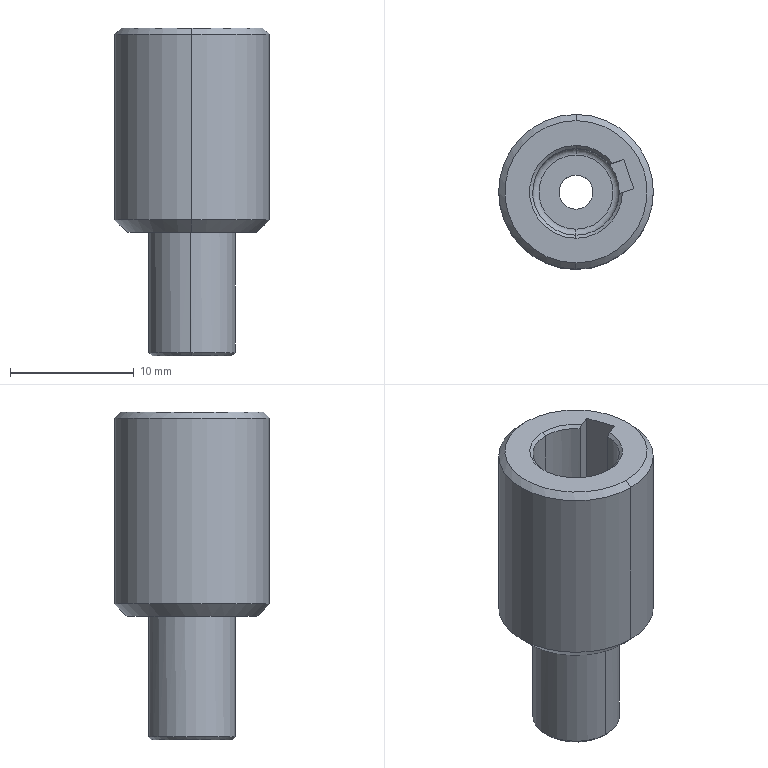Part | STEP file | 2026.6.15-Main Assembly图.sldasm-Part-128 | 1 solid | 37 faces | box 12.5 x 12.5 x 26.5 mm | volume 1705 mm3 | cylinder 13 | cone 11 | plane 11 | torus 2 | commonest cylinder face diameters 7 x5 2.5 x4 2.75 x2 12.5 x2
STEP:
#1=CARTESIAN_POINT('',(-1588.479,1436.224,3697.571));
#2=VERTEX_POINT('',#1);
#3=CARTESIAN_POINT('',(-1588.478,1436.235,3697.405));
#4=VERTEX_POINT('',#3);
#5=CARTESIAN_POINT('',(-1588.479,1436.224,3697.571));
#6=CARTESIAN_POINT('',(-1588.479,1436.224,3697.515));
#7=CARTESIAN_POINT('',(-1588.479,1436.228,3697.46));
#8=CARTESIAN_POINT('',(-1588.478,1436.235,3697.405));
#9=B_SPLINE_CURVE_WITH_KNOTS('',3,(#5,#6,#7,#8),.UNSPECIFIED.,.F.,.F.,(4,4),(0.,0.000165),.UNSPECIFIED.);
#10=EDGE_CURVE('',#2,#4,#9,.T.);
#11=ORIENTED_EDGE('',*,*,#10,.T.);
#12=CARTESIAN_POINT('',(-1589.685,1435.828,3697.405));
#13=VERTEX_POINT('',#12);
#14=CARTESIAN_POINT('',(-1589.685,1435.828,3697.405));
#15=DIRECTION('',(-0.9474,-0.3199,0.));
#16=VECTOR('',#15,1000.);
#17=LINE('',#14,#16);
#18=EDGE_CURVE('',#4,#13,#17,.T.);
#19=ORIENTED_EDGE('',*,*,#18,.T.);
#20=CARTESIAN_POINT('',(-1589.681,1435.818,3697.571));
#21=VERTEX_POINT('',#20);
#22=CARTESIAN_POINT('',(-1590.081,1437.002,3697.571));
#23=DIRECTION('',(0.9474,0.3199,0.));
#24=DIRECTION('',(-0.3171,0.9391,0.1324));
#25=AXIS2_PLACEMENT_3D('',#22,#23,#24);
#26=CIRCLE('',#25,1.25);
#27=EDGE_CURVE('',#21,#13,#26,.T.);
#28=ORIENTED_EDGE('',*,*,#27,.F.);
#29=CARTESIAN_POINT('',(-1589.681,1435.818,3697.571));
#30=DIRECTION('',(-0.9474,-0.3199,0.));
#31=VECTOR('',#30,1000.);
#32=LINE('',#29,#31);
#33=EDGE_CURVE('',#2,#21,#32,.T.);
#34=ORIENTED_EDGE('',*,*,#33,.F.);
#35=EDGE_LOOP('',(#11,#19,#28,#34));
#36=FACE_OUTER_BOUND('',#35,.T.);
#37=CARTESIAN_POINT('',(-1590.081,1437.002,3697.571));
#38=DIRECTION('',(-0.9474,-0.3199,0.));
#39=DIRECTION('',(0.3171,-0.9391,-0.1324));
#40=AXIS2_PLACEMENT_3D('',#37,#38,#39);
#41=CYLINDRICAL_SURFACE('',#40,1.25);
#42=ADVANCED_FACE('',(#36),#41,.F.);
#43=CARTESIAN_POINT('',(-1590.478,1438.176,3704.986));
#44=VERTEX_POINT('',#43);
#45=CARTESIAN_POINT('',(-1589.681,1435.818,3704.821));
#46=VERTEX_POINT('',#45);
#47=CARTESIAN_POINT('',(-1590.081,1437.002,3704.821));
#48=DIRECTION('',(0.9474,0.3199,0.));
#49=DIRECTION('',(-0.3171,0.9391,0.1324));
#50=AXIS2_PLACEMENT_3D('',#47,#48,#49);
#51=CIRCLE('',#50,1.25);
#52=EDGE_CURVE('',#44,#46,#51,.T.);
#53=ORIENTED_EDGE('',*,*,#52,.F.);
#54=CARTESIAN_POINT('',(-1589.271,1438.583,3704.986));
#55=VERTEX_POINT('',#54);
#56=CARTESIAN_POINT('',(-1590.478,1438.176,3704.986));
#57=DIRECTION('',(0.9474,0.3199,0.));
#58=VECTOR('',#57,1000.);
#59=LINE('',#56,#58);
#60=EDGE_CURVE('',#44,#55,#59,.T.);
#61=ORIENTED_EDGE('',*,*,#60,.T.);
#62=CARTESIAN_POINT('',(-1588.66,1437.482,3706.071));
#63=VERTEX_POINT('',#62);
#64=CARTESIAN_POINT('',(-1589.271,1438.583,3704.986));
#65=CARTESIAN_POINT('',(-1589.258,1438.567,3705.135));
#66=CARTESIAN_POINT('',(-1589.225,1438.527,3705.282));
#67=CARTESIAN_POINT('',(-1589.136,1438.409,3705.544));
#68=CARTESIAN_POINT('',(-1589.078,1438.328,3705.663));
#69=CARTESIAN_POINT('',(-1588.956,1438.134,3705.858));
#70=CARTESIAN_POINT('',(-1588.89,1438.019,3705.937));
#71=CARTESIAN_POINT('',(-1588.767,1437.765,3706.043));
#72=CARTESIAN_POINT('',(-1588.708,1437.625,3706.071));
#73=CARTESIAN_POINT('',(-1588.66,1437.482,3706.071));
#74=B_SPLINE_CURVE_WITH_KNOTS('',3,(#64,#65,#66,#67,#68,#69,#70,#71,#72,#73),.UNSPECIFIED.,.F.,.F.,(4,2,2,2,4),(0.000165,0.0006165,0.001068,0.001519,0.001971),.UNSPECIFIED.);
#75=EDGE_CURVE('',#55,#63,#74,.T.);
#76=ORIENTED_EDGE('',*,*,#75,.T.);
#77=CARTESIAN_POINT('',(-1588.479,1436.224,3704.821));
#78=VERTEX_POINT('',#77);
#79=CARTESIAN_POINT('',(-1588.66,1437.482,3706.071));
#80=CARTESIAN_POINT('',(-1588.634,1437.404,3706.071));
#81=CARTESIAN_POINT('',(-1588.61,1437.324,3706.062));
#82=CARTESIAN_POINT('',(-1588.569,1437.168,3706.03));
#83=CARTESIAN_POINT('',(-1588.552,1437.091,3706.006));
#84=CARTESIAN_POINT('',(-1588.509,1436.865,3705.911));
#85=CARTESIAN_POINT('',(-1588.493,1436.726,3705.819));
#86=CARTESIAN_POINT('',(-1588.481,1436.549,3705.647));
#87=CARTESIAN_POINT('',(-1588.478,1436.495,3705.585));
#88=CARTESIAN_POINT('',(-1588.476,1436.401,3705.45));
#89=CARTESIAN_POINT('',(-1588.476,1436.359,3705.377));
#90=CARTESIAN_POINT('',(-1588.477,1436.26,3705.152));
#91=CARTESIAN_POINT('',(-1588.479,1436.224,3704.987));
#92=CARTESIAN_POINT('',(-1588.479,1436.224,3704.821));
#93=B_SPLINE_CURVE_WITH_KNOTS('',3,(#79,#80,#81,#82,#83,#84,#85,#86,#87,#88,#89,#90,#91,#92),.UNSPECIFIED.,.F.,.F.,(4,2,2,2,2,2,4),(0.001971,0.002217,0.002463,0.002955,0.003201,0.003447,0.003939),.UNSPECIFIED.);
#94=EDGE_CURVE('',#63,#78,#93,.T.);
#95=ORIENTED_EDGE('',*,*,#94,.T.);
#96=CARTESIAN_POINT('',(-1589.681,1435.818,3704.821));
#97=DIRECTION('',(0.9474,0.3199,0.));
#98=VECTOR('',#97,1000.);
#99=LINE('',#96,#98);
#100=EDGE_CURVE('',#46,#78,#99,.T.);
#101=ORIENTED_EDGE('',*,*,#100,.F.);
#102=EDGE_LOOP('',(#53,#61,#76,#95,#101));
#103=FACE_OUTER_BOUND('',#102,.T.);
#104=CARTESIAN_POINT('',(-1590.081,1437.002,3704.821));
#105=DIRECTION('',(0.9474,0.3199,0.));
#106=DIRECTION('',(-0.3171,0.9391,0.1324));
#107=AXIS2_PLACEMENT_3D('',#104,#105,#106);
#108=CYLINDRICAL_SURFACE('',#107,1.25);
#109=ADVANCED_FACE('',(#103),#108,.F.);
#110=CARTESIAN_POINT('',(-1591.973,1439.862,3722.321));
#111=VERTEX_POINT('',#110);
#112=CARTESIAN_POINT('',(-1591.979,1432.862,3722.321));
#113=VERTEX_POINT('',#112);
#114=CARTESIAN_POINT('',(-1591.976,1436.362,3722.321));
#115=DIRECTION('',(0.,0.,1.));
#116=DIRECTION('',(0.0007664,1.,0.));
#117=AXIS2_PLACEMENT_3D('',#114,#115,#116);
#118=CIRCLE('',#117,3.5);
#119=EDGE_CURVE('',#111,#113,#118,.T.);
#120=ORIENTED_EDGE('',*,*,#119,.F.);
#121=CARTESIAN_POINT('',(-1591.973,1440.112,3722.571));
#122=VERTEX_POINT('',#121);
#123=CARTESIAN_POINT('',(-1591.973,1439.862,3722.321));
#124=DIRECTION('',(0.000542,0.7071,0.7071));
#125=VECTOR('',#124,1000.);
#126=LINE('',#123,#125);
#127=EDGE_CURVE('',#111,#122,#126,.T.);
#128=ORIENTED_EDGE('',*,*,#127,.T.);
#129=CARTESIAN_POINT('',(-1591.979,1432.612,3722.571));
#130=VERTEX_POINT('',#129);
#131=CARTESIAN_POINT('',(-1591.976,1436.362,3722.571));
#132=DIRECTION('',(0.,0.,-1.));
#133=DIRECTION('',(0.0007664,1.,0.));
#134=AXIS2_PLACEMENT_3D('',#131,#132,#133);
#135=CIRCLE('',#134,3.75);
#136=EDGE_CURVE('',#130,#122,#135,.T.);
#137=ORIENTED_EDGE('',*,*,#136,.F.);
#138=CARTESIAN_POINT('',(-1591.979,1432.862,3722.321));
#139=DIRECTION('',(-0.000542,-0.7071,0.7071));
#140=VECTOR('',#139,1000.);
#141=LINE('',#138,#140);
#142=EDGE_CURVE('',#113,#130,#141,.T.);
#143=ORIENTED_EDGE('',*,*,#142,.F.);
#144=EDGE_LOOP('',(#120,#128,#137,#143));
#145=FACE_OUTER_BOUND('',#144,.T.);
#146=CARTESIAN_POINT('',(-1591.976,1436.362,3722.321));
#147=DIRECTION('',(0.,0.,1.));
#148=DIRECTION('',(-0.0007664,-1.,0.));
#149=AXIS2_PLACEMENT_3D('',#146,#147,#148);
#150=CONICAL_SURFACE('',#149,3.5,0.7854);
#151=ADVANCED_FACE('',(#145),#150,.F.);
#152=CARTESIAN_POINT('',(-1588.479,1436.224,3722.321));
#153=VERTEX_POINT('',#152);
#154=CARTESIAN_POINT('',(-1591.976,1436.362,3722.321));
#155=DIRECTION('',(0.,0.,1.));
#156=DIRECTION('',(0.0007664,1.,0.));
#157=AXIS2_PLACEMENT_3D('',#154,#155,#156);
#158=CIRCLE('',#157,3.5);
#159=EDGE_CURVE('',#113,#153,#158,.T.);
#160=ORIENTED_EDGE('',*,*,#159,.F.);
#161=ORIENTED_EDGE('',*,*,#142,.T.);
#162=CARTESIAN_POINT('',(-1588.227,1436.309,3722.571));
#163=VERTEX_POINT('',#162);
#164=CARTESIAN_POINT('',(-1591.976,1436.362,3722.571));
#165=DIRECTION('',(0.,0.,-1.));
#166=DIRECTION('',(0.0007664,1.,0.));
#167=AXIS2_PLACEMENT_3D('',#164,#165,#166);
#168=CIRCLE('',#167,3.75);
#169=EDGE_CURVE('',#163,#130,#168,.T.);
#170=ORIENTED_EDGE('',*,*,#169,.F.);
#171=CARTESIAN_POINT('',(-1588.479,1436.224,3722.321));
#172=CARTESIAN_POINT('',(-1588.395,1436.252,3722.404));
#173=CARTESIAN_POINT('',(-1588.31,1436.281,3722.487));
#174=CARTESIAN_POINT('',(-1588.227,1436.309,3722.571));
#175=B_SPLINE_CURVE_WITH_KNOTS('',3,(#171,#172,#173,#174),.UNSPECIFIED.,.F.,.F.,(4,4),(0.,0.0003653),.UNSPECIFIED.);
#176=EDGE_CURVE('',#153,#163,#175,.T.);
#177=ORIENTED_EDGE('',*,*,#176,.F.);
#178=EDGE_LOOP('',(#160,#161,#170,#177));
#179=FACE_OUTER_BOUND('',#178,.T.);
#180=CARTESIAN_POINT('',(-1591.976,1436.362,3722.321));
#181=DIRECTION('',(0.,0.,1.));
#182=DIRECTION('',(-0.0007664,-1.,0.));
#183=AXIS2_PLACEMENT_3D('',#180,#181,#182);
#184=CONICAL_SURFACE('',#183,3.5,0.7854);
#185=ADVANCED_FACE('',(#179),#184,.F.);
#186=CARTESIAN_POINT('',(-1591.974,1439.612,3696.071));
#187=VERTEX_POINT('',#186);
#188=CARTESIAN_POINT('',(-1591.979,1433.112,3696.071));
#189=VERTEX_POINT('',#188);
#190=CARTESIAN_POINT('',(-1591.976,1436.362,3696.071));
#191=DIRECTION('',(0.,0.,-1.));
#192=DIRECTION('',(0.0007664,1.,0.));
#193=AXIS2_PLACEMENT_3D('',#190,#191,#192);
#194=CIRCLE('',#193,3.25);
#195=EDGE_CURVE('',#187,#189,#194,.T.);
#196=ORIENTED_EDGE('',*,*,#195,.F.);
#197=CARTESIAN_POINT('',(-1591.973,1439.862,3696.321));
#198=VERTEX_POINT('',#197);
#199=CARTESIAN_POINT('',(-1591.973,1439.862,3696.321));
#200=DIRECTION('',(0.000542,0.7071,0.7071));
#201=VECTOR('',#200,1000.);
#202=LINE('',#199,#201);
#203=EDGE_CURVE('',#187,#198,#202,.T.);
#204=ORIENTED_EDGE('',*,*,#203,.T.);
#205=CARTESIAN_POINT('',(-1591.84,1439.859,3696.321));
#206=VERTEX_POINT('',#205);
#207=CARTESIAN_POINT('',(-1591.976,1436.362,3696.321));
#208=DIRECTION('',(0.,0.,1.));
#209=DIRECTION('',(0.0007664,1.,0.));
#210=AXIS2_PLACEMENT_3D('',#207,#208,#209);
#211=CIRCLE('',#210,3.5);
#212=EDGE_CURVE('',#206,#198,#211,.T.);
#213=ORIENTED_EDGE('',*,*,#212,.F.);
#214=CARTESIAN_POINT('',(-1588.66,1437.482,3696.321));
#215=VERTEX_POINT('',#214);
#216=CARTESIAN_POINT('',(-1591.976,1436.362,3696.321));
#217=DIRECTION('',(0.,0.,1.));
#218=DIRECTION('',(0.0007664,1.,0.));
#219=AXIS2_PLACEMENT_3D('',#216,#217,#218);
#220=CIRCLE('',#219,3.5);
#221=EDGE_CURVE('',#215,#206,#220,.T.);
#222=ORIENTED_EDGE('',*,*,#221,.F.);
#223=CARTESIAN_POINT('',(-1591.979,1432.862,3696.321));
#224=VERTEX_POINT('',#223);
#225=CARTESIAN_POINT('',(-1591.976,1436.362,3696.321));
#226=DIRECTION('',(0.,0.,1.));
#227=DIRECTION('',(0.0007664,1.,0.));
#228=AXIS2_PLACEMENT_3D('',#225,#226,#227);
#229=CIRCLE('',#228,3.5);
#230=EDGE_CURVE('',#224,#215,#229,.T.);
#231=ORIENTED_EDGE('',*,*,#230,.F.);
#232=CARTESIAN_POINT('',(-1591.979,1432.862,3696.321));
#233=DIRECTION('',(-0.000542,-0.7071,0.7071));
#234=VECTOR('',#233,1000.);
#235=LINE('',#232,#234);
#236=EDGE_CURVE('',#189,#224,#235,.T.);
#237=ORIENTED_EDGE('',*,*,#236,.F.);
#238=EDGE_LOOP('',(#196,#204,#213,#222,#231,#237));
#239=FACE_OUTER_BOUND('',#238,.T.);
#240=CARTESIAN_POINT('',(-1591.976,1436.362,3696.321));
#241=DIRECTION('',(0.,0.,1.));
#242=DIRECTION('',(-0.0007664,-1.,0.));
#243=AXIS2_PLACEMENT_3D('',#240,#241,#242);
#244=CONICAL_SURFACE('',#243,3.5,0.7854);
#245=ADVANCED_FACE('',(#239),#244,.T.);
#246=CARTESIAN_POINT('',(-1591.977,1434.987,3696.321));
#247=VERTEX_POINT('',#246);
#248=CARTESIAN_POINT('',(-1591.975,1437.737,3696.321));
#249=VERTEX_POINT('',#248);
#250=CARTESIAN_POINT('',(-1591.976,1436.362,3696.321));
#251=DIRECTION('',(0.,0.,-1.));
#252=DIRECTION('',(0.0007664,1.,0.));
#253=AXIS2_PLACEMENT_3D('',#250,#251,#252);
#254=CIRCLE('',#253,1.375);
#255=EDGE_CURVE('',#247,#249,#254,.T.);
#256=ORIENTED_EDGE('',*,*,#255,.F.);
#257=CARTESIAN_POINT('',(-1591.977,1434.737,3696.071));
#258=VERTEX_POINT('',#257);
#259=CARTESIAN_POINT('',(-1591.977,1434.737,3696.071));
#260=DIRECTION('',(-0.000542,-0.7071,-0.7071));
#261=VECTOR('',#260,1000.);
#262=LINE('',#259,#261);
#263=EDGE_CURVE('',#247,#258,#262,.T.);
#264=ORIENTED_EDGE('',*,*,#263,.T.);
#265=CARTESIAN_POINT('',(-1591.975,1437.987,3696.071));
#266=VERTEX_POINT('',#265);
#267=CARTESIAN_POINT('',(-1591.976,1436.362,3696.071));
#268=DIRECTION('',(0.,0.,1.));
#269=DIRECTION('',(0.0007664,1.,0.));
#270=AXIS2_PLACEMENT_3D('',#267,#268,#269);
#271=CIRCLE('',#270,1.625);
#272=EDGE_CURVE('',#266,#258,#271,.T.);
#273=ORIENTED_EDGE('',*,*,#272,.F.);
#274=CARTESIAN_POINT('',(-1591.975,1437.987,3696.071));
#275=DIRECTION('',(0.000542,0.7071,-0.7071));
#276=VECTOR('',#275,1000.);
#277=LINE('',#274,#276);
#278=EDGE_CURVE('',#249,#266,#277,.T.);
#279=ORIENTED_EDGE('',*,*,#278,.F.);
#280=EDGE_LOOP('',(#256,#264,#273,#279));
#281=FACE_OUTER_BOUND('',#280,.T.);
#282=CARTESIAN_POINT('',(-1591.976,1436.362,3696.071));
#283=DIRECTION('',(0.,0.,-1.));
#284=DIRECTION('',(0.0007664,1.,0.));
#285=AXIS2_PLACEMENT_3D('',#282,#283,#284);
#286=CONICAL_SURFACE('',#285,1.625,0.7854);
#287=ADVANCED_FACE('',(#281),#286,.F.);
#288=CARTESIAN_POINT('',(-1591.981,1430.612,3722.571));
#289=VERTEX_POINT('',#288);
#290=CARTESIAN_POINT('',(-1591.972,1442.112,3722.571));
#291=VERTEX_POINT('',#290);
#292=CARTESIAN_POINT('',(-1591.976,1436.362,3722.571));
#293=DIRECTION('',(0.,0.,1.));
#294=DIRECTION('',(0.0007664,1.,0.));
#295=AXIS2_PLACEMENT_3D('',#292,#293,#294);
#296=CIRCLE('',#295,5.75);
#297=EDGE_CURVE('',#289,#291,#296,.T.);
#298=ORIENTED_EDGE('',*,*,#297,.F.);
#299=CARTESIAN_POINT('',(-1591.981,1430.112,3722.071));
#300=VERTEX_POINT('',#299);
#301=CARTESIAN_POINT('',(-1591.981,1430.112,3722.071));
#302=DIRECTION('',(-0.000542,-0.7071,-0.7071));
#303=VECTOR('',#302,1000.);
#304=LINE('',#301,#303);
#305=EDGE_CURVE('',#289,#300,#304,.T.);
#306=ORIENTED_EDGE('',*,*,#305,.T.);
#307=CARTESIAN_POINT('',(-1591.971,1442.612,3722.071));
#308=VERTEX_POINT('',#307);
#309=CARTESIAN_POINT('',(-1591.976,1436.362,3722.071));
#310=DIRECTION('',(0.,0.,-1.));
#311=DIRECTION('',(0.0007664,1.,0.));
#312=AXIS2_PLACEMENT_3D('',#309,#310,#311);
#313=CIRCLE('',#312,6.25);
#314=EDGE_CURVE('',#308,#300,#313,.T.);
#315=ORIENTED_EDGE('',*,*,#314,.F.);
#316=CARTESIAN_POINT('',(-1591.971,1442.612,3722.071));
#317=DIRECTION('',(0.000542,0.7071,-0.7071));
#318=VECTOR('',#317,1000.);
#319=LINE('',#316,#318);
#320=EDGE_CURVE('',#291,#308,#319,.T.);
#321=ORIENTED_EDGE('',*,*,#320,.F.);
#322=EDGE_LOOP('',(#298,#306,#315,#321));
#323=FACE_OUTER_BOUND('',#322,.T.);
#324=CARTESIAN_POINT('',(-1591.976,1436.362,3722.071));
#325=DIRECTION('',(0.,0.,-1.));
#326=DIRECTION('',(0.0007664,1.,0.));
#327=AXIS2_PLACEMENT_3D('',#324,#325,#326);
#328=CONICAL_SURFACE('',#327,6.25,0.7854);
#329=ADVANCED_FACE('',(#323),#328,.T.);
#330=CARTESIAN_POINT('',(-1591.972,1441.612,3706.071));
#331=VERTEX_POINT('',#330);
#332=CARTESIAN_POINT('',(-1591.98,1431.112,3706.071));
#333=VERTEX_POINT('',#332);
#334=CARTESIAN_POINT('',(-1591.976,1436.362,3706.071));
#335=DIRECTION('',(0.,0.,-1.));
#336=DIRECTION('',(0.0007664,1.,0.));
#337=AXIS2_PLACEMENT_3D('',#334,#335,#336);
#338=CIRCLE('',#337,5.25);
#339=EDGE_CURVE('',#331,#333,#338,.T.);
#340=ORIENTED_EDGE('',*,*,#339,.F.);
#341=CARTESIAN_POINT('',(-1591.971,1442.612,3707.071));
#342=VERTEX_POINT('',#341);
#343=CARTESIAN_POINT('',(-1591.972,1441.612,3706.071));
#344=DIRECTION('',(0.000542,0.7071,0.7071));
#345=VECTOR('',#344,1000.);
#346=LINE('',#343,#345);
#347=EDGE_CURVE('',#331,#342,#346,.T.);
#348=ORIENTED_EDGE('',*,*,#347,.T.);
#349=CARTESIAN_POINT('',(-1591.981,1430.112,3707.071));
#350=VERTEX_POINT('',#349);
#351=CARTESIAN_POINT('',(-1591.976,1436.362,3707.071));
#352=DIRECTION('',(0.,0.,1.));
#353=DIRECTION('',(0.0007664,1.,0.));
#354=AXIS2_PLACEMENT_3D('',#351,#352,#353);
#355=CIRCLE('',#354,6.25);
#356=EDGE_CURVE('',#350,#342,#355,.T.);
#357=ORIENTED_EDGE('',*,*,#356,.F.);
#358=CARTESIAN_POINT('',(-1591.98,1431.112,3706.071));
#359=DIRECTION('',(-0.000542,-0.7071,0.7071));
#360=VECTOR('',#359,1000.);
#361=LINE('',#358,#360);
#362=EDGE_CURVE('',#333,#350,#361,.T.);
#363=ORIENTED_EDGE('',*,*,#362,.F.);
#364=EDGE_LOOP('',(#340,#348,#357,#363));
#365=FACE_OUTER_BOUND('',#364,.T.);
#366=CARTESIAN_POINT('',(-1591.976,1436.362,3706.071));
#367=DIRECTION('',(0.,0.,1.));
#368=DIRECTION('',(-0.0007664,-1.,0.));
#369=AXIS2_PLACEMENT_3D('',#366,#367,#368);
#370=CONICAL_SURFACE('',#369,5.25,0.7854);
#371=ADVANCED_FACE('',(#365),#370,.T.);
#372=ORIENTED_EDGE('',*,*,#255,.T.);
#373=CARTESIAN_POINT('',(-1591.975,1437.737,3708.571));
#374=VERTEX_POINT('',#373);
#375=CARTESIAN_POINT('',(-1591.975,1437.737,3693.071));
#376=DIRECTION('',(0.,0.,1.));
#377=VECTOR('',#376,1000.);
#378=LINE('',#375,#377);
#379=EDGE_CURVE('',#249,#374,#378,.T.);
#380=ORIENTED_EDGE('',*,*,#379,.T.);
#381=CARTESIAN_POINT('',(-1591.977,1434.987,3708.571));
#382=VERTEX_POINT('',#381);
#383=CARTESIAN_POINT('',(-1591.976,1436.362,3708.571));
#384=DIRECTION('',(0.,0.,-1.));
#385=DIRECTION('',(-0.0007664,-1.,0.));
#386=AXIS2_PLACEMENT_3D('',#383,#384,#385);
#387=CIRCLE('',#386,1.375);
#388=EDGE_CURVE('',#382,#374,#387,.T.);
#389=ORIENTED_EDGE('',*,*,#388,.F.);
#390=CARTESIAN_POINT('',(-1591.977,1434.987,3693.071));
#391=DIRECTION('',(0.,0.,1.));
#392=VECTOR('',#391,1000.);
#393=LINE('',#390,#392);
#394=EDGE_CURVE('',#247,#382,#393,.T.);
#395=ORIENTED_EDGE('',*,*,#394,.F.);
#396=EDGE_LOOP('',(#372,#380,#389,#395));
#397=FACE_OUTER_BOUND('',#396,.T.);
#398=CARTESIAN_POINT('',(-1591.976,1436.362,3693.071));
#399=DIRECTION('',(0.,0.,1.));
#400=DIRECTION('',(-0.0007664,-1.,0.));
#401=AXIS2_PLACEMENT_3D('',#398,#399,#400);
#402=CYLINDRICAL_SURFACE('',#401,1.375);
#403=ADVANCED_FACE('',(#397),#402,.F.);
#404=CARTESIAN_POINT('',(-1591.974,1439.362,3708.571));
#405=VERTEX_POINT('',#404);
#406=CARTESIAN_POINT('',(-1591.978,1433.362,3708.571));
#407=VERTEX_POINT('',#406);
#408=CARTESIAN_POINT('',(-1591.976,1436.362,3708.571));
#409=DIRECTION('',(0.,0.,1.));
#410=DIRECTION('',(-0.0007664,-1.,0.));
#411=AXIS2_PLACEMENT_3D('',#408,#409,#410);
#412=CIRCLE('',#411,3.);
#413=EDGE_CURVE('',#405,#407,#412,.T.);
#414=ORIENTED_EDGE('',*,*,#413,.F.);
#415=CARTESIAN_POINT('',(-1591.973,1439.862,3709.071));
#416=VERTEX_POINT('',#415);
#417=CARTESIAN_POINT('',(-1591.974,1439.362,3709.071));
#418=DIRECTION('',(1.,-0.0007664,0.));
#419=DIRECTION('',(0.0007664,1.,0.));
#420=AXIS2_PLACEMENT_3D('',#417,#418,#419);
#421=CIRCLE('',#420,0.5);
#422=EDGE_CURVE('',#405,#416,#421,.T.);
#423=ORIENTED_EDGE('',*,*,#422,.T.);
#424=CARTESIAN_POINT('',(-1591.979,1432.862,3709.071));
#425=VERTEX_POINT('',#424);
#426=CARTESIAN_POINT('',(-1591.976,1436.362,3709.071));
#427=DIRECTION('',(0.,0.,-1.));
#428=DIRECTION('',(-0.0007664,-1.,0.));
#429=AXIS2_PLACEMENT_3D('',#426,#427,#428);
#430=CIRCLE('',#429,3.5);
#431=EDGE_CURVE('',#425,#416,#430,.T.);
#432=ORIENTED_EDGE('',*,*,#431,.F.);
#433=CARTESIAN_POINT('',(-1591.978,1433.362,3709.071));
#434=DIRECTION('',(-1.,0.0007664,0.));
#435=DIRECTION('',(-0.0007664,-1.,0.));
#436=AXIS2_PLACEMENT_3D('',#433,#434,#435);
#437=CIRCLE('',#436,0.5);
#438=EDGE_CURVE('',#407,#425,#437,.T.);
#439=ORIENTED_EDGE('',*,*,#438,.F.);
#440=EDGE_LOOP('',(#414,#423,#432,#439));
#441=FACE_OUTER_BOUND('',#440,.T.);
#442=CARTESIAN_POINT('',(-1591.976,1436.362,3709.071));
#443=DIRECTION('',(0.,0.,1.));
#444=DIRECTION('',(-0.0007664,-1.,0.));
#445=AXIS2_PLACEMENT_3D('',#442,#443,#444);
#446=TOROIDAL_SURFACE('',#445,3.,0.5);
#447=ADVANCED_FACE('',(#441),#446,.F.);
#448=ORIENTED_EDGE('',*,*,#431,.T.);
#449=CARTESIAN_POINT('',(-1591.973,1439.862,3708.571));
#450=DIRECTION('',(0.,0.,1.));
#451=VECTOR('',#450,1000.);
#452=LINE('',#449,#451);
#453=EDGE_CURVE('',#416,#111,#452,.T.);
#454=ORIENTED_EDGE('',*,*,#453,.T.);
#455=ORIENTED_EDGE('',*,*,#119,.T.);
#456=CARTESIAN_POINT('',(-1591.979,1432.862,3708.571));
#457=DIRECTION('',(0.,0.,1.));
#458=VECTOR('',#457,1000.);
#459=LINE('',#456,#458);
#460=EDGE_CURVE('',#425,#113,#459,.T.);
#461=ORIENTED_EDGE('',*,*,#460,.F.);
#462=EDGE_LOOP('',(#448,#454,#455,#461));
#463=FACE_OUTER_BOUND('',#462,.T.);
#464=CARTESIAN_POINT('',(-1591.976,1436.362,3708.571));
#465=DIRECTION('',(0.,0.,1.));
#466=DIRECTION('',(-0.0007664,-1.,0.));
#467=AXIS2_PLACEMENT_3D('',#464,#465,#466);
#468=CYLINDRICAL_SURFACE('',#467,3.5);
#469=ADVANCED_FACE('',(#463),#468,.F.);
#470=ORIENTED_EDGE('',*,*,#356,.T.);
#471=CARTESIAN_POINT('',(-1591.971,1442.612,3706.071));
#472=DIRECTION('',(0.,0.,1.));
#473=VECTOR('',#472,1000.);
#474=LINE('',#471,#473);
#475=EDGE_CURVE('',#342,#308,#474,.T.);
#476=ORIENTED_EDGE('',*,*,#475,.T.);
#477=ORIENTED_EDGE('',*,*,#314,.T.);
#478=CARTESIAN_POINT('',(-1591.981,1430.112,3706.071));
#479=DIRECTION('',(0.,0.,1.));
#480=VECTOR('',#479,1000.);
#481=LINE('',#478,#480);
#482=EDGE_CURVE('',#350,#300,#481,.T.);
#483=ORIENTED_EDGE('',*,*,#482,.F.);
#484=EDGE_LOOP('',(#470,#476,#477,#483));
#485=FACE_OUTER_BOUND('',#484,.T.);
#486=CARTESIAN_POINT('',(-1591.976,1436.362,3706.071));
#487=DIRECTION('',(0.,0.,1.));
#488=DIRECTION('',(-0.0007664,-1.,0.));
#489=AXIS2_PLACEMENT_3D('',#486,#487,#488);
#490=CYLINDRICAL_SURFACE('',#489,6.25);
#491=ADVANCED_FACE('',(#485),#490,.T.);
#492=CARTESIAN_POINT('',(-1592.112,1432.865,3706.071));
#493=VERTEX_POINT('',#492);
#494=CARTESIAN_POINT('',(-1591.976,1436.362,3706.071));
#495=DIRECTION('',(0.,0.,-1.));
#496=DIRECTION('',(0.03892,0.9992,0.));
#497=AXIS2_PLACEMENT_3D('',#494,#495,#496);
#498=CIRCLE('',#497,3.5);
#499=EDGE_CURVE('',#63,#493,#498,.T.);
#500=ORIENTED_EDGE('',*,*,#499,.T.);
#501=CARTESIAN_POINT('',(-1592.112,1432.865,3696.321));
#502=VERTEX_POINT('',#501);
#503=CARTESIAN_POINT('',(-1592.112,1432.865,3706.071));
#504=DIRECTION('',(0.,0.,-1.));
#505=VECTOR('',#504,1000.);
#506=LINE('',#503,#505);
#507=EDGE_CURVE('',#493,#502,#506,.T.);
#508=ORIENTED_EDGE('',*,*,#507,.T.);
#509=CARTESIAN_POINT('',(-1591.976,1436.362,3696.321));
#510=DIRECTION('',(0.,0.,1.));
#511=DIRECTION('',(0.0007664,1.,0.));
#512=AXIS2_PLACEMENT_3D('',#509,#510,#511);
#513=CIRCLE('',#512,3.5);
#514=EDGE_CURVE('',#502,#224,#513,.T.);
#515=ORIENTED_EDGE('',*,*,#514,.T.);
#516=ORIENTED_EDGE('',*,*,#230,.T.);
#517=CARTESIAN_POINT('',(-1588.478,1436.235,3697.405));
#518=CARTESIAN_POINT('',(-1588.478,1436.257,3697.256));
#519=CARTESIAN_POINT('',(-1588.476,1436.308,3697.11));
#520=CARTESIAN_POINT('',(-1588.477,1436.456,3696.848));
#521=CARTESIAN_POINT('',(-1588.48,1436.555,3696.729));
#522=CARTESIAN_POINT('',(-1588.5,1436.784,3696.533));
#523=CARTESIAN_POINT('',(-1588.517,1436.915,3696.455));
#524=CARTESIAN_POINT('',(-1588.573,1437.192,3696.349));
#525=CARTESIAN_POINT('',(-1588.612,1437.339,3696.321));
#526=CARTESIAN_POINT('',(-1588.66,1437.482,3696.321));
#527=B_SPLINE_CURVE_WITH_KNOTS('',3,(#517,#518,#519,#520,#521,#522,#523,#524,#525,#526),.UNSPECIFIED.,.F.,.F.,(4,2,2,2,4),(0.000165,0.0006165,0.001068,0.001519,0.001971),.UNSPECIFIED.);
#528=EDGE_CURVE('',#4,#215,#527,.T.);
#529=ORIENTED_EDGE('',*,*,#528,.F.);
#530=ORIENTED_EDGE('',*,*,#10,.F.);
#531=CARTESIAN_POINT('',(-1588.479,1436.224,3706.071));
#532=DIRECTION('',(0.,0.,-1.));
#533=VECTOR('',#532,1000.);
#534=LINE('',#531,#533);
#535=EDGE_CURVE('',#78,#2,#534,.T.);
#536=ORIENTED_EDGE('',*,*,#535,.F.);
#537=ORIENTED_EDGE('',*,*,#94,.F.);
#538=EDGE_LOOP('',(#500,#508,#515,#516,#529,#530,#536,#537));
#539=FACE_OUTER_BOUND('',#538,.T.);
#540=CARTESIAN_POINT('',(-1591.976,1436.362,3706.071));
#541=DIRECTION('',(0.,0.,-1.));
#542=DIRECTION('',(0.03892,0.9992,0.));
#543=AXIS2_PLACEMENT_3D('',#540,#541,#542);
#544=CYLINDRICAL_SURFACE('',#543,3.5);
#545=ADVANCED_FACE('',(#539),#544,.T.);
#546=ORIENTED_EDGE('',*,*,#507,.F.);
#547=CARTESIAN_POINT('',(-1591.84,1439.859,3706.071));
#548=VERTEX_POINT('',#547);
#549=CARTESIAN_POINT('',(-1591.976,1436.362,3706.071));
#550=DIRECTION('',(0.,0.,-1.));
#551=DIRECTION('',(0.03892,0.9992,0.));
#552=AXIS2_PLACEMENT_3D('',#549,#550,#551);
#553=CIRCLE('',#552,3.5);
#554=EDGE_CURVE('',#493,#548,#553,.T.);
#555=ORIENTED_EDGE('',*,*,#554,.T.);
#556=CARTESIAN_POINT('',(-1591.84,1439.859,3706.071));
#557=DIRECTION('',(0.,0.,-1.));
#558=VECTOR('',#557,1000.);
#559=LINE('',#556,#558);
#560=EDGE_CURVE('',#548,#206,#559,.T.);
#561=ORIENTED_EDGE('',*,*,#560,.T.);
#562=ORIENTED_EDGE('',*,*,#212,.T.);
#563=CARTESIAN_POINT('',(-1591.976,1436.362,3696.321));
#564=DIRECTION('',(0.,0.,1.));
#565=DIRECTION('',(0.0007664,1.,0.));
#566=AXIS2_PLACEMENT_3D('',#563,#564,#565);
#567=CIRCLE('',#566,3.5);
#568=EDGE_CURVE('',#198,#502,#567,.T.);
#569=ORIENTED_EDGE('',*,*,#568,.T.);
#570=EDGE_LOOP('',(#546,#555,#561,#562,#569));
#571=FACE_OUTER_BOUND('',#570,.T.);
#572=CARTESIAN_POINT('',(-1591.976,1436.362,3706.071));
#573=DIRECTION('',(0.,0.,-1.));
#574=DIRECTION('',(0.03892,0.9992,0.));
#575=AXIS2_PLACEMENT_3D('',#572,#573,#574);
#576=CYLINDRICAL_SURFACE('',#575,3.5);
#577=ADVANCED_FACE('',(#571),#576,.T.);
#578=ORIENTED_EDGE('',*,*,#272,.T.);
#579=CARTESIAN_POINT('',(-1591.976,1436.362,3696.071));
#580=DIRECTION('',(0.,0.,1.));
#581=DIRECTION('',(0.0007664,1.,0.));
#582=AXIS2_PLACEMENT_3D('',#579,#580,#581);
#583=CIRCLE('',#582,1.625);
#584=EDGE_CURVE('',#258,#266,#583,.T.);
#585=ORIENTED_EDGE('',*,*,#584,.T.);
#586=EDGE_LOOP('',(#578,#585));
#587=FACE_BOUND('',#586,.T.);
#588=CARTESIAN_POINT('',(-1591.976,1436.362,3696.071));
#589=DIRECTION('',(0.,0.,-1.));
#590=DIRECTION('',(0.0007664,1.,0.));
#591=AXIS2_PLACEMENT_3D('',#588,#589,#590);
#592=CIRCLE('',#591,3.25);
#593=EDGE_CURVE('',#189,#187,#592,.T.);
#594=ORIENTED_EDGE('',*,*,#593,.T.);
#595=ORIENTED_EDGE('',*,*,#195,.T.);
#596=EDGE_LOOP('',(#594,#595));
#597=FACE_OUTER_BOUND('',#596,.T.);
#598=CARTESIAN_POINT('',(-1591.976,1436.362,3696.071));
#599=DIRECTION('',(0.,0.,-1.));
#600=DIRECTION('',(0.0007664,1.,0.));
#601=AXIS2_PLACEMENT_3D('',#598,#599,#600);
#602=PLANE('',#601);
#603=ADVANCED_FACE('',(#587,#597),#602,.T.);
#604=ORIENTED_EDGE('',*,*,#560,.F.);
#605=CARTESIAN_POINT('',(-1591.976,1436.362,3706.071));
#606=DIRECTION('',(0.,0.,-1.));
#607=DIRECTION('',(0.03892,0.9992,0.));
#608=AXIS2_PLACEMENT_3D('',#605,#606,#607);
#609=CIRCLE('',#608,3.5);
#610=EDGE_CURVE('',#548,#63,#609,.T.);
#611=ORIENTED_EDGE('',*,*,#610,.T.);
#612=ORIENTED_EDGE('',*,*,#75,.F.);
#613=CARTESIAN_POINT('',(-1589.279,1438.592,3704.821));
#614=VERTEX_POINT('',#613);
#615=CARTESIAN_POINT('',(-1589.279,1438.592,3704.821));
#616=CARTESIAN_POINT('',(-1589.279,1438.592,3704.877));
#617=CARTESIAN_POINT('',(-1589.276,1438.589,3704.932));
#618=CARTESIAN_POINT('',(-1589.271,1438.583,3704.986));
#619=B_SPLINE_CURVE_WITH_KNOTS('',3,(#615,#616,#617,#618),.UNSPECIFIED.,.F.,.F.,(4,4),(0.,0.000165),.UNSPECIFIED.);
#620=EDGE_CURVE('',#614,#55,#619,.T.);
#621=ORIENTED_EDGE('',*,*,#620,.F.);
#622=CARTESIAN_POINT('',(-1589.279,1438.592,3697.571));
#623=VERTEX_POINT('',#622);
#624=CARTESIAN_POINT('',(-1589.279,1438.592,3706.071));
#625=DIRECTION('',(0.,0.,1.));
#626=VECTOR('',#625,1000.);
#627=LINE('',#624,#626);
#628=EDGE_CURVE('',#623,#614,#627,.T.);
#629=ORIENTED_EDGE('',*,*,#628,.F.);
#630=CARTESIAN_POINT('',(-1588.66,1437.482,3696.321));
#631=CARTESIAN_POINT('',(-1588.686,1437.56,3696.321));
#632=CARTESIAN_POINT('',(-1588.716,1437.638,3696.329));
#633=CARTESIAN_POINT('',(-1588.778,1437.787,3696.361));
#634=CARTESIAN_POINT('',(-1588.811,1437.858,3696.385));
#635=CARTESIAN_POINT('',(-1588.914,1438.064,3696.48));
#636=CARTESIAN_POINT('',(-1588.985,1438.184,3696.572));
#637=CARTESIAN_POINT('',(-1589.083,1438.333,3696.745));
#638=CARTESIAN_POINT('',(-1589.114,1438.377,3696.807));
#639=CARTESIAN_POINT('',(-1589.169,1438.453,3696.942));
#640=CARTESIAN_POINT('',(-1589.194,1438.486,3697.015));
#641=CARTESIAN_POINT('',(-1589.255,1438.565,3697.24));
#642=CARTESIAN_POINT('',(-1589.279,1438.592,3697.404));
#643=CARTESIAN_POINT('',(-1589.279,1438.592,3697.571));
#644=B_SPLINE_CURVE_WITH_KNOTS('',3,(#630,#631,#632,#633,#634,#635,#636,#637,#638,#639,#640,#641,#642,#643),.UNSPECIFIED.,.F.,.F.,(4,2,2,2,2,2,4),(0.001971,0.002217,0.002463,0.002955,0.003201,0.003447,0.003939),.UNSPECIFIED.);
#645=EDGE_CURVE('',#215,#623,#644,.T.);
#646=ORIENTED_EDGE('',*,*,#645,.F.);
#647=ORIENTED_EDGE('',*,*,#221,.T.);
#648=EDGE_LOOP('',(#604,#611,#612,#621,#629,#646,#647));
#649=FACE_OUTER_BOUND('',#648,.T.);
#650=CARTESIAN_POINT('',(-1591.976,1436.362,3706.071));
#651=DIRECTION('',(0.,0.,-1.));
#652=DIRECTION('',(0.03892,0.9992,0.));
#653=AXIS2_PLACEMENT_3D('',#650,#651,#652);
#654=CYLINDRICAL_SURFACE('',#653,3.5);
#655=ADVANCED_FACE('',(#649),#654,.T.);
#656=ORIENTED_EDGE('',*,*,#475,.F.);
#657=CARTESIAN_POINT('',(-1591.976,1436.362,3707.071));
#658=DIRECTION('',(0.,0.,1.));
#659=DIRECTION('',(0.0007664,1.,0.));
#660=AXIS2_PLACEMENT_3D('',#657,#658,#659);
#661=CIRCLE('',#660,6.25);
#662=EDGE_CURVE('',#342,#350,#661,.T.);
#663=ORIENTED_EDGE('',*,*,#662,.T.);
#664=ORIENTED_EDGE('',*,*,#482,.T.);
#665=CARTESIAN_POINT('',(-1591.976,1436.362,3722.071));
#666=DIRECTION('',(0.,0.,-1.));
#667=DIRECTION('',(0.0007664,1.,0.));
#668=AXIS2_PLACEMENT_3D('',#665,#666,#667);
#669=CIRCLE('',#668,6.25);
#670=EDGE_CURVE('',#300,#308,#669,.T.);
#671=ORIENTED_EDGE('',*,*,#670,.T.);
#672=EDGE_LOOP('',(#656,#663,#664,#671));
#673=FACE_OUTER_BOUND('',#672,.T.);
#674=CARTESIAN_POINT('',(-1591.976,1436.362,3706.071));
#675=DIRECTION('',(0.,0.,1.));
#676=DIRECTION('',(-0.0007664,-1.,0.));
#677=AXIS2_PLACEMENT_3D('',#674,#675,#676);
#678=CYLINDRICAL_SURFACE('',#677,6.25);
#679=ADVANCED_FACE('',(#673),#678,.T.);
#680=CARTESIAN_POINT('',(-1591.976,1436.362,3706.071));
#681=DIRECTION('',(0.,0.,-1.));
#682=DIRECTION('',(0.0007664,1.,0.));
#683=AXIS2_PLACEMENT_3D('',#680,#681,#682);
#684=CIRCLE('',#683,5.25);
#685=EDGE_CURVE('',#333,#331,#684,.T.);
#686=ORIENTED_EDGE('',*,*,#685,.T.);
#687=ORIENTED_EDGE('',*,*,#339,.T.);
#688=EDGE_LOOP('',(#686,#687));
#689=FACE_OUTER_BOUND('',#688,.T.);
#690=ORIENTED_EDGE('',*,*,#499,.F.);
#691=ORIENTED_EDGE('',*,*,#610,.F.);
#692=ORIENTED_EDGE('',*,*,#554,.F.);
#693=EDGE_LOOP('',(#690,#691,#692));
#694=FACE_BOUND('',#693,.T.);
#695=CARTESIAN_POINT('',(-1591.976,1436.362,3706.071));
#696=DIRECTION('',(0.,0.,-1.));
#697=DIRECTION('',(0.0007664,1.,0.));
#698=AXIS2_PLACEMENT_3D('',#695,#696,#697);
#699=PLANE('',#698);
#700=ADVANCED_FACE('',(#689,#694),#699,.T.);
#701=CARTESIAN_POINT('',(-1591.976,1436.362,3722.571));
#702=DIRECTION('',(0.,0.,1.));
#703=DIRECTION('',(0.0007664,1.,0.));
#704=AXIS2_PLACEMENT_3D('',#701,#702,#703);
#705=CIRCLE('',#704,5.75);
#706=EDGE_CURVE('',#291,#289,#705,.T.);
#707=ORIENTED_EDGE('',*,*,#706,.T.);
#708=ORIENTED_EDGE('',*,*,#297,.T.);
#709=EDGE_LOOP('',(#707,#708));
#710=FACE_OUTER_BOUND('',#709,.T.);
#711=CARTESIAN_POINT('',(-1587.313,1436.617,3722.571));
#712=VERTEX_POINT('',#711);
#713=CARTESIAN_POINT('',(-1587.313,1436.617,3722.571));
#714=DIRECTION('',(-0.9474,-0.3199,0.));
#715=VECTOR('',#714,1000.);
#716=LINE('',#713,#715);
#717=EDGE_CURVE('',#712,#163,#716,.T.);
#718=ORIENTED_EDGE('',*,*,#717,.T.);
#719=ORIENTED_EDGE('',*,*,#169,.T.);
#720=ORIENTED_EDGE('',*,*,#136,.T.);
#721=CARTESIAN_POINT('',(-1589.026,1438.677,3722.571));
#722=VERTEX_POINT('',#721);
#723=CARTESIAN_POINT('',(-1591.976,1436.362,3722.571));
#724=DIRECTION('',(0.,0.,-1.));
#725=DIRECTION('',(0.0007664,1.,0.));
#726=AXIS2_PLACEMENT_3D('',#723,#724,#725);
#727=CIRCLE('',#726,3.75);
#728=EDGE_CURVE('',#122,#722,#727,.T.);
#729=ORIENTED_EDGE('',*,*,#728,.T.);
#730=CARTESIAN_POINT('',(-1588.113,1438.986,3722.571));
#731=VERTEX_POINT('',#730);
#732=CARTESIAN_POINT('',(-1589.279,1438.592,3722.571));
#733=DIRECTION('',(0.9474,0.3199,0.));
#734=VECTOR('',#733,1000.);
#735=LINE('',#732,#734);
#736=EDGE_CURVE('',#722,#731,#735,.T.);
#737=ORIENTED_EDGE('',*,*,#736,.T.);
#738=CARTESIAN_POINT('',(-1588.113,1438.986,3722.571));
#739=DIRECTION('',(0.3199,-0.9474,0.));
#740=VECTOR('',#739,1000.);
#741=LINE('',#738,#740);
#742=EDGE_CURVE('',#731,#712,#741,.T.);
#743=ORIENTED_EDGE('',*,*,#742,.T.);
#744=EDGE_LOOP('',(#718,#719,#720,#729,#737,#743));
#745=FACE_BOUND('',#744,.T.);
#746=CARTESIAN_POINT('',(-1591.976,1436.362,3722.571));
#747=DIRECTION('',(0.,0.,-1.));
#748=DIRECTION('',(0.0007664,1.,0.));
#749=AXIS2_PLACEMENT_3D('',#746,#747,#748);
#750=PLANE('',#749);
#751=ADVANCED_FACE('',(#710,#745),#750,.F.);
#752=ORIENTED_EDGE('',*,*,#453,.F.);
#753=CARTESIAN_POINT('',(-1591.976,1436.362,3709.071));
#754=DIRECTION('',(0.,0.,-1.));
#755=DIRECTION('',(-0.0007664,-1.,0.));
#756=AXIS2_PLACEMENT_3D('',#753,#754,#755);
#757=CIRCLE('',#756,3.5);
#758=EDGE_CURVE('',#416,#425,#757,.T.);
#759=ORIENTED_EDGE('',*,*,#758,.T.);
#760=ORIENTED_EDGE('',*,*,#460,.T.);
#761=ORIENTED_EDGE('',*,*,#159,.T.);
#762=CARTESIAN_POINT('',(-1588.479,1436.224,3709.571));
#763=VERTEX_POINT('',#762);
#764=CARTESIAN_POINT('',(-1588.479,1436.224,3709.571));
#765=DIRECTION('',(0.,0.,1.));
#766=VECTOR('',#765,1000.);
#767=LINE('',#764,#766);
#768=EDGE_CURVE('',#763,#153,#767,.T.);
#769=ORIENTED_EDGE('',*,*,#768,.F.);
#770=CARTESIAN_POINT('',(-1589.279,1438.592,3709.571));
#771=VERTEX_POINT('',#770);
#772=CARTESIAN_POINT('',(-1591.976,1436.362,3709.571));
#773=DIRECTION('',(0.,0.,1.));
#774=DIRECTION('',(-0.3199,0.9474,0.));
#775=AXIS2_PLACEMENT_3D('',#772,#773,#774);
#776=CIRCLE('',#775,3.5);
#777=EDGE_CURVE('',#763,#771,#776,.T.);
#778=ORIENTED_EDGE('',*,*,#777,.T.);
#779=CARTESIAN_POINT('',(-1589.279,1438.592,3722.321));
#780=VERTEX_POINT('',#779);
#781=CARTESIAN_POINT('',(-1589.279,1438.592,3709.571));
#782=DIRECTION('',(0.,0.,1.));
#783=VECTOR('',#782,1000.);
#784=LINE('',#781,#783);
#785=EDGE_CURVE('',#771,#780,#784,.T.);
#786=ORIENTED_EDGE('',*,*,#785,.T.);
#787=CARTESIAN_POINT('',(-1591.976,1436.362,3722.321));
#788=DIRECTION('',(0.,0.,1.));
#789=DIRECTION('',(0.0007664,1.,0.));
#790=AXIS2_PLACEMENT_3D('',#787,#788,#789);
#791=CIRCLE('',#790,3.5);
#792=EDGE_CURVE('',#780,#111,#791,.T.);
#793=ORIENTED_EDGE('',*,*,#792,.T.);
#794=EDGE_LOOP('',(#752,#759,#760,#761,#769,#778,#786,#793));
#795=FACE_OUTER_BOUND('',#794,.T.);
#796=CARTESIAN_POINT('',(-1591.976,1436.362,3708.571));
#797=DIRECTION('',(0.,0.,1.));
#798=DIRECTION('',(-0.0007664,-1.,0.));
#799=AXIS2_PLACEMENT_3D('',#796,#797,#798);
#800=CYLINDRICAL_SURFACE('',#799,3.5);
#801=ADVANCED_FACE('',(#795),#800,.F.);
#802=ORIENTED_EDGE('',*,*,#388,.T.);
#803=CARTESIAN_POINT('',(-1591.976,1436.362,3708.571));
#804=DIRECTION('',(0.,0.,-1.));
#805=DIRECTION('',(-0.0007664,-1.,0.));
#806=AXIS2_PLACEMENT_3D('',#803,#804,#805);
#807=CIRCLE('',#806,1.375);
#808=EDGE_CURVE('',#374,#382,#807,.T.);
#809=ORIENTED_EDGE('',*,*,#808,.T.);
#810=EDGE_LOOP('',(#802,#809));
#811=FACE_BOUND('',#810,.T.);
#812=CARTESIAN_POINT('',(-1591.976,1436.362,3708.571));
#813=DIRECTION('',(0.,0.,1.));
#814=DIRECTION('',(-0.0007664,-1.,0.));
#815=AXIS2_PLACEMENT_3D('',#812,#813,#814);
#816=CIRCLE('',#815,3.);
#817=EDGE_CURVE('',#407,#405,#816,.T.);
#818=ORIENTED_EDGE('',*,*,#817,.T.);
#819=ORIENTED_EDGE('',*,*,#413,.T.);
#820=EDGE_LOOP('',(#818,#819));
#821=FACE_OUTER_BOUND('',#820,.T.);
#822=CARTESIAN_POINT('',(-1591.976,1436.362,3708.571));
#823=DIRECTION('',(0.,0.,1.));
#824=DIRECTION('',(-0.0007664,-1.,0.));
#825=AXIS2_PLACEMENT_3D('',#822,#823,#824);
#826=PLANE('',#825);
#827=ADVANCED_FACE('',(#811,#821),#826,.T.);
#828=ORIENTED_EDGE('',*,*,#736,.F.);
#829=CARTESIAN_POINT('',(-1589.026,1438.677,3722.571));
#830=CARTESIAN_POINT('',(-1589.11,1438.649,3722.487));
#831=CARTESIAN_POINT('',(-1589.194,1438.621,3722.404));
#832=CARTESIAN_POINT('',(-1589.279,1438.592,3722.321));
#833=B_SPLINE_CURVE_WITH_KNOTS('',3,(#829,#830,#831,#832),.UNSPECIFIED.,.F.,.F.,(4,4),(0.,0.0003653),.UNSPECIFIED.);
#834=EDGE_CURVE('',#722,#780,#833,.T.);
#835=ORIENTED_EDGE('',*,*,#834,.T.);
#836=ORIENTED_EDGE('',*,*,#785,.F.);
#837=CARTESIAN_POINT('',(-1588.113,1438.986,3709.571));
#838=VERTEX_POINT('',#837);
#839=CARTESIAN_POINT('',(-1589.279,1438.592,3709.571));
#840=DIRECTION('',(-0.9474,-0.3199,0.));
#841=VECTOR('',#840,1000.);
#842=LINE('',#839,#841);
#843=EDGE_CURVE('',#838,#771,#842,.T.);
#844=ORIENTED_EDGE('',*,*,#843,.F.);
#845=CARTESIAN_POINT('',(-1588.113,1438.986,3709.571));
#846=DIRECTION('',(0.,0.,-1.));
#847=VECTOR('',#846,1000.);
#848=LINE('',#845,#847);
#849=EDGE_CURVE('',#731,#838,#848,.T.);
#850=ORIENTED_EDGE('',*,*,#849,.F.);
#851=EDGE_LOOP('',(#828,#835,#836,#844,#850));
#852=FACE_OUTER_BOUND('',#851,.T.);
#853=CARTESIAN_POINT('',(-1589.279,1438.592,3709.571));
#854=DIRECTION('',(0.3199,-0.9474,0.));
#855=DIRECTION('',(0.9474,0.3199,0.009787));
#856=AXIS2_PLACEMENT_3D('',#853,#854,#855);
#857=PLANE('',#856);
#858=ADVANCED_FACE('',(#852),#857,.T.);
#859=ORIENTED_EDGE('',*,*,#742,.F.);
#860=ORIENTED_EDGE('',*,*,#849,.T.);
#861=CARTESIAN_POINT('',(-1587.313,1436.617,3709.571));
#862=VERTEX_POINT('',#861);
#863=CARTESIAN_POINT('',(-1588.113,1438.986,3709.571));
#864=DIRECTION('',(-0.3199,0.9474,0.));
#865=VECTOR('',#864,1000.);
#866=LINE('',#863,#865);
#867=EDGE_CURVE('',#862,#838,#866,.T.);
#868=ORIENTED_EDGE('',*,*,#867,.F.);
#869=CARTESIAN_POINT('',(-1587.313,1436.617,3709.571));
#870=DIRECTION('',(0.,0.,-1.));
#871=VECTOR('',#870,1000.);
#872=LINE('',#869,#871);
#873=EDGE_CURVE('',#712,#862,#872,.T.);
#874=ORIENTED_EDGE('',*,*,#873,.F.);
#875=EDGE_LOOP('',(#859,#860,#868,#874));
#876=FACE_OUTER_BOUND('',#875,.T.);
#877=CARTESIAN_POINT('',(-1588.113,1438.986,3709.571));
#878=DIRECTION('',(-0.9474,-0.3199,0.));
#879=DIRECTION('',(0.3171,-0.9391,-0.1324));
#880=AXIS2_PLACEMENT_3D('',#877,#878,#879);
#881=PLANE('',#880);
#882=ADVANCED_FACE('',(#876),#881,.T.);
#883=ORIENTED_EDGE('',*,*,#768,.T.);
#884=ORIENTED_EDGE('',*,*,#176,.T.);
#885=ORIENTED_EDGE('',*,*,#717,.F.);
#886=ORIENTED_EDGE('',*,*,#873,.T.);
#887=CARTESIAN_POINT('',(-1587.313,1436.617,3709.571));
#888=DIRECTION('',(0.9474,0.3199,0.));
#889=VECTOR('',#888,1000.);
#890=LINE('',#887,#889);
#891=EDGE_CURVE('',#763,#862,#890,.T.);
#892=ORIENTED_EDGE('',*,*,#891,.F.);
#893=EDGE_LOOP('',(#883,#884,#885,#886,#892));
#894=FACE_OUTER_BOUND('',#893,.T.);
#895=CARTESIAN_POINT('',(-1587.313,1436.617,3709.571));
#896=DIRECTION('',(-0.3199,0.9474,0.));
#897=DIRECTION('',(-0.9474,-0.3199,-0.009787));
#898=AXIS2_PLACEMENT_3D('',#895,#896,#897);
#899=PLANE('',#898);
#900=ADVANCED_FACE('',(#894),#899,.T.);
#901=ORIENTED_EDGE('',*,*,#843,.T.);
#902=ORIENTED_EDGE('',*,*,#777,.F.);
#903=ORIENTED_EDGE('',*,*,#891,.T.);
#904=ORIENTED_EDGE('',*,*,#867,.T.);
#905=EDGE_LOOP('',(#901,#902,#903,#904));
#906=FACE_OUTER_BOUND('',#905,.T.);
#907=CARTESIAN_POINT('',(-1591.976,1436.362,3709.571));
#908=DIRECTION('',(0.,0.,1.));
#909=DIRECTION('',(-0.0007664,-1.,0.));
#910=AXIS2_PLACEMENT_3D('',#907,#908,#909);
#911=PLANE('',#910);
#912=ADVANCED_FACE('',(#906),#911,.T.);
#913=ORIENTED_EDGE('',*,*,#422,.F.);
#914=ORIENTED_EDGE('',*,*,#817,.F.);
#915=ORIENTED_EDGE('',*,*,#438,.T.);
#916=ORIENTED_EDGE('',*,*,#758,.F.);
#917=EDGE_LOOP('',(#913,#914,#915,#916));
#918=FACE_OUTER_BOUND('',#917,.T.);
#919=CARTESIAN_POINT('',(-1591.976,1436.362,3709.071));
#920=DIRECTION('',(0.,0.,1.));
#921=DIRECTION('',(-0.0007664,-1.,0.));
#922=AXIS2_PLACEMENT_3D('',#919,#920,#921);
#923=TOROIDAL_SURFACE('',#922,3.,0.5);
#924=ADVANCED_FACE('',(#918),#923,.F.);
#925=ORIENTED_EDGE('',*,*,#379,.F.);
#926=CARTESIAN_POINT('',(-1591.976,1436.362,3696.321));
#927=DIRECTION('',(0.,0.,-1.));
#928=DIRECTION('',(0.0007664,1.,0.));
#929=AXIS2_PLACEMENT_3D('',#926,#927,#928);
#930=CIRCLE('',#929,1.375);
#931=EDGE_CURVE('',#249,#247,#930,.T.);
#932=ORIENTED_EDGE('',*,*,#931,.T.);
#933=ORIENTED_EDGE('',*,*,#394,.T.);
#934=ORIENTED_EDGE('',*,*,#808,.F.);
#935=EDGE_LOOP('',(#925,#932,#933,#934));
#936=FACE_OUTER_BOUND('',#935,.T.);
#937=CARTESIAN_POINT('',(-1591.976,1436.362,3693.071));
#938=DIRECTION('',(0.,0.,1.));
#939=DIRECTION('',(-0.0007664,-1.,0.));
#940=AXIS2_PLACEMENT_3D('',#937,#938,#939);
#941=CYLINDRICAL_SURFACE('',#940,1.375);
#942=ADVANCED_FACE('',(#936),#941,.F.);
#943=ORIENTED_EDGE('',*,*,#347,.F.);
#944=ORIENTED_EDGE('',*,*,#685,.F.);
#945=ORIENTED_EDGE('',*,*,#362,.T.);
#946=ORIENTED_EDGE('',*,*,#662,.F.);
#947=EDGE_LOOP('',(#943,#944,#945,#946));
#948=FACE_OUTER_BOUND('',#947,.T.);
#949=CARTESIAN_POINT('',(-1591.976,1436.362,3706.071));
#950=DIRECTION('',(0.,0.,1.));
#951=DIRECTION('',(-0.0007664,-1.,0.));
#952=AXIS2_PLACEMENT_3D('',#949,#950,#951);
#953=CONICAL_SURFACE('',#952,5.25,0.7854);
#954=ADVANCED_FACE('',(#948),#953,.T.);
#955=ORIENTED_EDGE('',*,*,#305,.F.);
#956=ORIENTED_EDGE('',*,*,#706,.F.);
#957=ORIENTED_EDGE('',*,*,#320,.T.);
#958=ORIENTED_EDGE('',*,*,#670,.F.);
#959=EDGE_LOOP('',(#955,#956,#957,#958));
#960=FACE_OUTER_BOUND('',#959,.T.);
#961=CARTESIAN_POINT('',(-1591.976,1436.362,3722.071));
#962=DIRECTION('',(0.,0.,-1.));
#963=DIRECTION('',(0.0007664,1.,0.));
#964=AXIS2_PLACEMENT_3D('',#961,#962,#963);
#965=CONICAL_SURFACE('',#964,6.25,0.7854);
#966=ADVANCED_FACE('',(#960),#965,.T.);
#967=ORIENTED_EDGE('',*,*,#263,.F.);
#968=ORIENTED_EDGE('',*,*,#931,.F.);
#969=ORIENTED_EDGE('',*,*,#278,.T.);
#970=ORIENTED_EDGE('',*,*,#584,.F.);
#971=EDGE_LOOP('',(#967,#968,#969,#970));
#972=FACE_OUTER_BOUND('',#971,.T.);
#973=CARTESIAN_POINT('',(-1591.976,1436.362,3696.071));
#974=DIRECTION('',(0.,0.,-1.));
#975=DIRECTION('',(0.0007664,1.,0.));
#976=AXIS2_PLACEMENT_3D('',#973,#974,#975);
#977=CONICAL_SURFACE('',#976,1.625,0.7854);
#978=ADVANCED_FACE('',(#972),#977,.F.);
#979=ORIENTED_EDGE('',*,*,#203,.F.);
#980=ORIENTED_EDGE('',*,*,#593,.F.);
#981=ORIENTED_EDGE('',*,*,#236,.T.);
#982=ORIENTED_EDGE('',*,*,#514,.F.);
#983=ORIENTED_EDGE('',*,*,#568,.F.);
#984=EDGE_LOOP('',(#979,#980,#981,#982,#983));
#985=FACE_OUTER_BOUND('',#984,.T.);
#986=CARTESIAN_POINT('',(-1591.976,1436.362,3696.321));
#987=DIRECTION('',(0.,0.,1.));
#988=DIRECTION('',(-0.0007664,-1.,0.));
#989=AXIS2_PLACEMENT_3D('',#986,#987,#988);
#990=CONICAL_SURFACE('',#989,3.5,0.7854);
#991=ADVANCED_FACE('',(#985),#990,.T.);
#992=ORIENTED_EDGE('',*,*,#127,.F.);
#993=ORIENTED_EDGE('',*,*,#792,.F.);
#994=ORIENTED_EDGE('',*,*,#834,.F.);
#995=ORIENTED_EDGE('',*,*,#728,.F.);
#996=EDGE_LOOP('',(#992,#993,#994,#995));
#997=FACE_OUTER_BOUND('',#996,.T.);
#998=CARTESIAN_POINT('',(-1591.976,1436.362,3722.321));
#999=DIRECTION('',(0.,0.,1.));
#1000=DIRECTION('',(-0.0007664,-1.,0.));
#1001=AXIS2_PLACEMENT_3D('',#998,#999,#1000);
#1002=CONICAL_SURFACE('',#1001,3.5,0.7854);
#1003=ADVANCED_FACE('',(#997),#1002,.F.);
#1004=ORIENTED_EDGE('',*,*,#535,.T.);
#1005=ORIENTED_EDGE('',*,*,#33,.T.);
#1006=CARTESIAN_POINT('',(-1589.681,1435.818,3706.071));
#1007=DIRECTION('',(0.,0.,1.));
#1008=VECTOR('',#1007,1000.);
#1009=LINE('',#1006,#1008);
#1010=EDGE_CURVE('',#21,#46,#1009,.T.);
#1011=ORIENTED_EDGE('',*,*,#1010,.T.);
#1012=ORIENTED_EDGE('',*,*,#100,.T.);
#1013=EDGE_LOOP('',(#1004,#1005,#1011,#1012));
#1014=FACE_OUTER_BOUND('',#1013,.T.);
#1015=CARTESIAN_POINT('',(-1589.681,1435.818,3706.071));
#1016=DIRECTION('',(0.3199,-0.9474,0.));
#1017=DIRECTION('',(0.,0.,-1.));
#1018=AXIS2_PLACEMENT_3D('',#1015,#1016,#1017);
#1019=PLANE('',#1018);
#1020=ADVANCED_FACE('',(#1014),#1019,.F.);
#1021=ORIENTED_EDGE('',*,*,#628,.T.);
#1022=CARTESIAN_POINT('',(-1590.481,1438.186,3704.821));
#1023=VERTEX_POINT('',#1022);
#1024=CARTESIAN_POINT('',(-1590.481,1438.186,3704.821));
#1025=DIRECTION('',(-0.9474,-0.3199,0.));
#1026=VECTOR('',#1025,1000.);
#1027=LINE('',#1024,#1026);
#1028=EDGE_CURVE('',#614,#1023,#1027,.T.);
#1029=ORIENTED_EDGE('',*,*,#1028,.T.);
#1030=CARTESIAN_POINT('',(-1590.481,1438.186,3697.571));
#1031=VERTEX_POINT('',#1030);
#1032=CARTESIAN_POINT('',(-1590.481,1438.186,3706.071));
#1033=DIRECTION('',(0.,0.,1.));
#1034=VECTOR('',#1033,1000.);
#1035=LINE('',#1032,#1034);
#1036=EDGE_CURVE('',#1031,#1023,#1035,.T.);
#1037=ORIENTED_EDGE('',*,*,#1036,.F.);
#1038=CARTESIAN_POINT('',(-1590.481,1438.186,3697.571));
#1039=DIRECTION('',(0.9474,0.3199,0.));
#1040=VECTOR('',#1039,1000.);
#1041=LINE('',#1038,#1040);
#1042=EDGE_CURVE('',#1031,#623,#1041,.T.);
#1043=ORIENTED_EDGE('',*,*,#1042,.T.);
#1044=EDGE_LOOP('',(#1021,#1029,#1037,#1043));
#1045=FACE_OUTER_BOUND('',#1044,.T.);
#1046=CARTESIAN_POINT('',(-1590.481,1438.186,3706.071));
#1047=DIRECTION('',(0.3199,-0.9474,0.));
#1048=DIRECTION('',(0.,0.,-1.));
#1049=AXIS2_PLACEMENT_3D('',#1046,#1047,#1048);
#1050=PLANE('',#1049);
#1051=ADVANCED_FACE('',(#1045),#1050,.T.);
#1052=ORIENTED_EDGE('',*,*,#1010,.F.);
#1053=ORIENTED_EDGE('',*,*,#27,.T.);
#1054=CARTESIAN_POINT('',(-1590.081,1437.002,3697.571));
#1055=DIRECTION('',(0.9474,0.3199,0.));
#1056=DIRECTION('',(-0.3171,0.9391,0.1324));
#1057=AXIS2_PLACEMENT_3D('',#1054,#1055,#1056);
#1058=CIRCLE('',#1057,1.25);
#1059=EDGE_CURVE('',#13,#1031,#1058,.T.);
#1060=ORIENTED_EDGE('',*,*,#1059,.T.);
#1061=ORIENTED_EDGE('',*,*,#1036,.T.);
#1062=CARTESIAN_POINT('',(-1590.081,1437.002,3704.821));
#1063=DIRECTION('',(0.9474,0.3199,0.));
#1064=DIRECTION('',(-0.3171,0.9391,0.1324));
#1065=AXIS2_PLACEMENT_3D('',#1062,#1063,#1064);
#1066=CIRCLE('',#1065,1.25);
#1067=EDGE_CURVE('',#1023,#44,#1066,.T.);
#1068=ORIENTED_EDGE('',*,*,#1067,.T.);
#1069=ORIENTED_EDGE('',*,*,#52,.T.);
#1070=EDGE_LOOP('',(#1052,#1053,#1060,#1061,#1068,#1069));
#1071=FACE_OUTER_BOUND('',#1070,.T.);
#1072=CARTESIAN_POINT('',(-1589.681,1435.818,3706.071));
#1073=DIRECTION('',(0.9474,0.3199,0.));
#1074=DIRECTION('',(-0.3171,0.9391,0.1324));
#1075=AXIS2_PLACEMENT_3D('',#1072,#1073,#1074);
#1076=PLANE('',#1075);
#1077=ADVANCED_FACE('',(#1071),#1076,.T.);
#1078=ORIENTED_EDGE('',*,*,#60,.F.);
#1079=ORIENTED_EDGE('',*,*,#1067,.F.);
#1080=ORIENTED_EDGE('',*,*,#1028,.F.);
#1081=ORIENTED_EDGE('',*,*,#620,.T.);
#1082=EDGE_LOOP('',(#1078,#1079,#1080,#1081));
#1083=FACE_OUTER_BOUND('',#1082,.T.);
#1084=CARTESIAN_POINT('',(-1590.081,1437.002,3704.821));
#1085=DIRECTION('',(0.9474,0.3199,0.));
#1086=DIRECTION('',(-0.3171,0.9391,0.1324));
#1087=AXIS2_PLACEMENT_3D('',#1084,#1085,#1086);
#1088=CYLINDRICAL_SURFACE('',#1087,1.25);
#1089=ADVANCED_FACE('',(#1083),#1088,.F.);
#1090=ORIENTED_EDGE('',*,*,#18,.F.);
#1091=ORIENTED_EDGE('',*,*,#528,.T.);
#1092=ORIENTED_EDGE('',*,*,#645,.T.);
#1093=ORIENTED_EDGE('',*,*,#1042,.F.);
#1094=ORIENTED_EDGE('',*,*,#1059,.F.);
#1095=EDGE_LOOP('',(#1090,#1091,#1092,#1093,#1094));
#1096=FACE_OUTER_BOUND('',#1095,.T.);
#1097=CARTESIAN_POINT('',(-1590.081,1437.002,3697.571));
#1098=DIRECTION('',(-0.9474,-0.3199,0.));
#1099=DIRECTION('',(0.3171,-0.9391,-0.1324));
#1100=AXIS2_PLACEMENT_3D('',#1097,#1098,#1099);
#1101=CYLINDRICAL_SURFACE('',#1100,1.25);
#1102=ADVANCED_FACE('',(#1096),#1101,.F.);
#1103=CLOSED_SHELL('',(#42,#109,#151,#185,#245,#287,#329,#371,#403,#447,#469,#491,#545,#577,#603,#655,#679,#700,#751,#801,#827,#858,#882,#900,#912,#924,#942,#954,#966,#978,#991,#1003,#1020,#1051,#1077,#1089,#1102));
#1104=MANIFOLD_SOLID_BREP('',#1103);
#1105=CARTESIAN_POINT('',(0.,0.,0.));
#1106=DIRECTION('',(0.,0.,1.));
#1107=DIRECTION('',(1.,0.,0.));
#1108=AXIS2_PLACEMENT_3D('',#1105,#1106,#1107);
#1109=(LENGTH_UNIT()NAMED_UNIT(*)SI_UNIT(.MILLI.,.METRE.));
#1110=UNCERTAINTY_MEASURE_WITH_UNIT(LENGTH_MEASURE(0.00001),#1109,'','');
#1111=(NAMED_UNIT(*)PLANE_ANGLE_UNIT()SI_UNIT($,.RADIAN.));
#1112=(NAMED_UNIT(*)SI_UNIT($,.STERADIAN.)SOLID_ANGLE_UNIT());
#1113=(GEOMETRIC_REPRESENTATION_CONTEXT(3)GLOBAL_UNCERTAINTY_ASSIGNED_CONTEXT((#1110))GLOBAL_UNIT_ASSIGNED_CONTEXT((#1109,#1111,#1112))REPRESENTATION_CONTEXT('',''));
#1114=ADVANCED_BREP_SHAPE_REPRESENTATION('',(#1104,#1108),#1113);